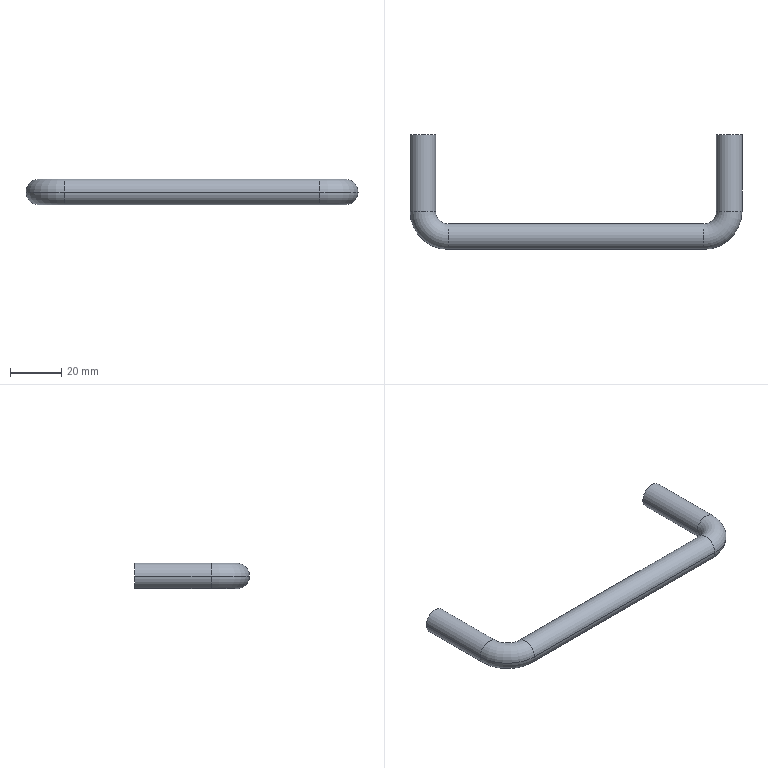Part | SolidWorks | features Sweep 1 | 1 solid | 12 faces | box 130 x 45 x 10 mm | volume 15034 mm3 | cylinder 6 | torus 4 | plane 2 | commonest cylinder face diameters 10 x6
STEP:
#1=CARTESIAN_POINT('',(50.,-5.,0.));
#2=VERTEX_POINT('',#1);
#3=CARTESIAN_POINT('',(50.,5.,0.));
#4=VERTEX_POINT('',#3);
#5=CARTESIAN_POINT('',(50.,0.,0.));
#6=DIRECTION('',(-1.,0.,0.));
#7=DIRECTION('',(0.,0.,-1.));
#8=AXIS2_PLACEMENT_3D('',#5,#6,#7);
#9=CIRCLE('',#8,5.);
#10=EDGE_CURVE('',#2,#4,#9,.T.);
#11=ORIENTED_EDGE('',*,*,#10,.F.);
#12=CARTESIAN_POINT('',(65.,10.,0.));
#13=VERTEX_POINT('',#12);
#14=CARTESIAN_POINT('',(50.,10.,0.));
#15=DIRECTION('',(0.,0.,1.));
#16=DIRECTION('',(1.,0.,0.));
#17=AXIS2_PLACEMENT_3D('',#14,#15,#16);
#18=CIRCLE('',#17,15.);
#19=EDGE_CURVE('',#2,#13,#18,.T.);
#20=ORIENTED_EDGE('',*,*,#19,.T.);
#21=CARTESIAN_POINT('',(55.,10.,0.));
#22=VERTEX_POINT('',#21);
#23=CARTESIAN_POINT('',(60.,10.,0.));
#24=DIRECTION('',(0.,-1.,0.));
#25=DIRECTION('',(0.,0.,-1.));
#26=AXIS2_PLACEMENT_3D('',#23,#24,#25);
#27=CIRCLE('',#26,5.);
#28=EDGE_CURVE('',#13,#22,#27,.T.);
#29=ORIENTED_EDGE('',*,*,#28,.T.);
#30=CARTESIAN_POINT('',(50.,10.,0.));
#31=DIRECTION('',(0.,0.,1.));
#32=DIRECTION('',(1.,0.,0.));
#33=AXIS2_PLACEMENT_3D('',#30,#31,#32);
#34=CIRCLE('',#33,5.);
#35=EDGE_CURVE('',#4,#22,#34,.T.);
#36=ORIENTED_EDGE('',*,*,#35,.F.);
#37=EDGE_LOOP('',(#11,#20,#29,#36));
#38=FACE_OUTER_BOUND('',#37,.T.);
#39=CARTESIAN_POINT('',(50.,10.,0.));
#40=DIRECTION('',(0.,0.,1.));
#41=DIRECTION('',(1.,0.,0.));
#42=AXIS2_PLACEMENT_3D('',#39,#40,#41);
#43=TOROIDAL_SURFACE('',#42,10.,5.);
#44=ADVANCED_FACE('',(#38),#43,.T.);
#45=CARTESIAN_POINT('',(-65.,10.,0.));
#46=VERTEX_POINT('',#45);
#47=CARTESIAN_POINT('',(-55.,10.,0.));
#48=VERTEX_POINT('',#47);
#49=CARTESIAN_POINT('',(-60.,10.,0.));
#50=DIRECTION('',(0.,1.,0.));
#51=DIRECTION('',(0.,0.,-1.));
#52=AXIS2_PLACEMENT_3D('',#49,#50,#51);
#53=CIRCLE('',#52,5.);
#54=EDGE_CURVE('',#46,#48,#53,.T.);
#55=ORIENTED_EDGE('',*,*,#54,.F.);
#56=CARTESIAN_POINT('',(-50.,-5.,0.));
#57=VERTEX_POINT('',#56);
#58=CARTESIAN_POINT('',(-50.,10.,0.));
#59=DIRECTION('',(0.,0.,1.));
#60=DIRECTION('',(1.,0.,0.));
#61=AXIS2_PLACEMENT_3D('',#58,#59,#60);
#62=CIRCLE('',#61,15.);
#63=EDGE_CURVE('',#46,#57,#62,.T.);
#64=ORIENTED_EDGE('',*,*,#63,.T.);
#65=CARTESIAN_POINT('',(-50.,5.,0.));
#66=VERTEX_POINT('',#65);
#67=CARTESIAN_POINT('',(-50.,0.,0.));
#68=DIRECTION('',(-1.,0.,0.));
#69=DIRECTION('',(0.,0.,-1.));
#70=AXIS2_PLACEMENT_3D('',#67,#68,#69);
#71=CIRCLE('',#70,5.);
#72=EDGE_CURVE('',#57,#66,#71,.T.);
#73=ORIENTED_EDGE('',*,*,#72,.T.);
#74=CARTESIAN_POINT('',(-50.,10.,0.));
#75=DIRECTION('',(0.,0.,1.));
#76=DIRECTION('',(1.,0.,0.));
#77=AXIS2_PLACEMENT_3D('',#74,#75,#76);
#78=CIRCLE('',#77,5.);
#79=EDGE_CURVE('',#48,#66,#78,.T.);
#80=ORIENTED_EDGE('',*,*,#79,.F.);
#81=EDGE_LOOP('',(#55,#64,#73,#80));
#82=FACE_OUTER_BOUND('',#81,.T.);
#83=CARTESIAN_POINT('',(-50.,10.,0.));
#84=DIRECTION('',(0.,0.,1.));
#85=DIRECTION('',(1.,0.,0.));
#86=AXIS2_PLACEMENT_3D('',#83,#84,#85);
#87=TOROIDAL_SURFACE('',#86,10.,5.);
#88=ADVANCED_FACE('',(#82),#87,.T.);
#89=ORIENTED_EDGE('',*,*,#28,.F.);
#90=CARTESIAN_POINT('',(65.,40.,0.));
#91=VERTEX_POINT('',#90);
#92=CARTESIAN_POINT('',(65.,10.,0.));
#93=DIRECTION('',(0.,1.,0.));
#94=VECTOR('',#93,1000.);
#95=LINE('',#92,#94);
#96=EDGE_CURVE('',#13,#91,#95,.T.);
#97=ORIENTED_EDGE('',*,*,#96,.T.);
#98=CARTESIAN_POINT('',(55.,40.,0.));
#99=VERTEX_POINT('',#98);
#100=CARTESIAN_POINT('',(60.,40.,0.));
#101=DIRECTION('',(0.,-1.,0.));
#102=DIRECTION('',(0.,0.,-1.));
#103=AXIS2_PLACEMENT_3D('',#100,#101,#102);
#104=CIRCLE('',#103,5.);
#105=EDGE_CURVE('',#91,#99,#104,.T.);
#106=ORIENTED_EDGE('',*,*,#105,.T.);
#107=CARTESIAN_POINT('',(55.,10.,0.));
#108=DIRECTION('',(0.,1.,0.));
#109=VECTOR('',#108,1000.);
#110=LINE('',#107,#109);
#111=EDGE_CURVE('',#22,#99,#110,.T.);
#112=ORIENTED_EDGE('',*,*,#111,.F.);
#113=EDGE_LOOP('',(#89,#97,#106,#112));
#114=FACE_OUTER_BOUND('',#113,.T.);
#115=CARTESIAN_POINT('',(60.,10.,0.));
#116=DIRECTION('',(0.,1.,0.));
#117=DIRECTION('',(-1.,0.,0.));
#118=AXIS2_PLACEMENT_3D('',#115,#116,#117);
#119=CYLINDRICAL_SURFACE('',#118,5.);
#120=ADVANCED_FACE('',(#114),#119,.T.);
#121=ORIENTED_EDGE('',*,*,#72,.F.);
#122=CARTESIAN_POINT('',(-50.,-5.,0.));
#123=DIRECTION('',(1.,0.,0.));
#124=VECTOR('',#123,1000.);
#125=LINE('',#122,#124);
#126=EDGE_CURVE('',#57,#2,#125,.T.);
#127=ORIENTED_EDGE('',*,*,#126,.T.);
#128=ORIENTED_EDGE('',*,*,#10,.T.);
#129=CARTESIAN_POINT('',(-50.,5.,0.));
#130=DIRECTION('',(1.,0.,0.));
#131=VECTOR('',#130,1000.);
#132=LINE('',#129,#131);
#133=EDGE_CURVE('',#66,#4,#132,.T.);
#134=ORIENTED_EDGE('',*,*,#133,.F.);
#135=EDGE_LOOP('',(#121,#127,#128,#134));
#136=FACE_OUTER_BOUND('',#135,.T.);
#137=CARTESIAN_POINT('',(-50.,0.,0.));
#138=DIRECTION('',(1.,0.,0.));
#139=DIRECTION('',(0.,1.,0.));
#140=AXIS2_PLACEMENT_3D('',#137,#138,#139);
#141=CYLINDRICAL_SURFACE('',#140,5.);
#142=ADVANCED_FACE('',(#136),#141,.T.);
#143=CARTESIAN_POINT('',(-65.,40.,0.));
#144=VERTEX_POINT('',#143);
#145=CARTESIAN_POINT('',(-55.,40.,0.));
#146=VERTEX_POINT('',#145);
#147=CARTESIAN_POINT('',(-60.,40.,0.));
#148=DIRECTION('',(0.,1.,0.));
#149=DIRECTION('',(0.,0.,-1.));
#150=AXIS2_PLACEMENT_3D('',#147,#148,#149);
#151=CIRCLE('',#150,5.);
#152=EDGE_CURVE('',#144,#146,#151,.T.);
#153=ORIENTED_EDGE('',*,*,#152,.F.);
#154=CARTESIAN_POINT('',(-65.,40.,0.));
#155=DIRECTION('',(0.,-1.,0.));
#156=VECTOR('',#155,1000.);
#157=LINE('',#154,#156);
#158=EDGE_CURVE('',#144,#46,#157,.T.);
#159=ORIENTED_EDGE('',*,*,#158,.T.);
#160=ORIENTED_EDGE('',*,*,#54,.T.);
#161=CARTESIAN_POINT('',(-55.,40.,0.));
#162=DIRECTION('',(0.,-1.,0.));
#163=VECTOR('',#162,1000.);
#164=LINE('',#161,#163);
#165=EDGE_CURVE('',#146,#48,#164,.T.);
#166=ORIENTED_EDGE('',*,*,#165,.F.);
#167=EDGE_LOOP('',(#153,#159,#160,#166));
#168=FACE_OUTER_BOUND('',#167,.T.);
#169=CARTESIAN_POINT('',(-60.,40.,0.));
#170=DIRECTION('',(0.,-1.,0.));
#171=DIRECTION('',(1.,0.,0.));
#172=AXIS2_PLACEMENT_3D('',#169,#170,#171);
#173=CYLINDRICAL_SURFACE('',#172,5.);
#174=ADVANCED_FACE('',(#168),#173,.T.);
#175=ORIENTED_EDGE('',*,*,#96,.F.);
#176=CARTESIAN_POINT('',(60.,10.,0.));
#177=DIRECTION('',(0.,-1.,0.));
#178=DIRECTION('',(0.,0.,-1.));
#179=AXIS2_PLACEMENT_3D('',#176,#177,#178);
#180=CIRCLE('',#179,5.);
#181=EDGE_CURVE('',#22,#13,#180,.T.);
#182=ORIENTED_EDGE('',*,*,#181,.F.);
#183=ORIENTED_EDGE('',*,*,#111,.T.);
#184=CARTESIAN_POINT('',(60.,40.,0.));
#185=DIRECTION('',(0.,-1.,0.));
#186=DIRECTION('',(0.,0.,-1.));
#187=AXIS2_PLACEMENT_3D('',#184,#185,#186);
#188=CIRCLE('',#187,5.);
#189=EDGE_CURVE('',#99,#91,#188,.T.);
#190=ORIENTED_EDGE('',*,*,#189,.T.);
#191=EDGE_LOOP('',(#175,#182,#183,#190));
#192=FACE_OUTER_BOUND('',#191,.T.);
#193=CARTESIAN_POINT('',(60.,10.,0.));
#194=DIRECTION('',(0.,1.,0.));
#195=DIRECTION('',(-1.,0.,0.));
#196=AXIS2_PLACEMENT_3D('',#193,#194,#195);
#197=CYLINDRICAL_SURFACE('',#196,5.);
#198=ADVANCED_FACE('',(#192),#197,.T.);
#199=ORIENTED_EDGE('',*,*,#19,.F.);
#200=CARTESIAN_POINT('',(50.,0.,0.));
#201=DIRECTION('',(-1.,0.,0.));
#202=DIRECTION('',(0.,0.,-1.));
#203=AXIS2_PLACEMENT_3D('',#200,#201,#202);
#204=CIRCLE('',#203,5.);
#205=EDGE_CURVE('',#4,#2,#204,.T.);
#206=ORIENTED_EDGE('',*,*,#205,.F.);
#207=ORIENTED_EDGE('',*,*,#35,.T.);
#208=ORIENTED_EDGE('',*,*,#181,.T.);
#209=EDGE_LOOP('',(#199,#206,#207,#208));
#210=FACE_OUTER_BOUND('',#209,.T.);
#211=CARTESIAN_POINT('',(50.,10.,0.));
#212=DIRECTION('',(0.,0.,1.));
#213=DIRECTION('',(1.,0.,0.));
#214=AXIS2_PLACEMENT_3D('',#211,#212,#213);
#215=TOROIDAL_SURFACE('',#214,10.,5.);
#216=ADVANCED_FACE('',(#210),#215,.T.);
#217=ORIENTED_EDGE('',*,*,#126,.F.);
#218=CARTESIAN_POINT('',(-50.,0.,0.));
#219=DIRECTION('',(-1.,0.,0.));
#220=DIRECTION('',(0.,0.,-1.));
#221=AXIS2_PLACEMENT_3D('',#218,#219,#220);
#222=CIRCLE('',#221,5.);
#223=EDGE_CURVE('',#66,#57,#222,.T.);
#224=ORIENTED_EDGE('',*,*,#223,.F.);
#225=ORIENTED_EDGE('',*,*,#133,.T.);
#226=ORIENTED_EDGE('',*,*,#205,.T.);
#227=EDGE_LOOP('',(#217,#224,#225,#226));
#228=FACE_OUTER_BOUND('',#227,.T.);
#229=CARTESIAN_POINT('',(-50.,0.,0.));
#230=DIRECTION('',(1.,0.,0.));
#231=DIRECTION('',(0.,1.,0.));
#232=AXIS2_PLACEMENT_3D('',#229,#230,#231);
#233=CYLINDRICAL_SURFACE('',#232,5.);
#234=ADVANCED_FACE('',(#228),#233,.T.);
#235=ORIENTED_EDGE('',*,*,#63,.F.);
#236=CARTESIAN_POINT('',(-60.,10.,0.));
#237=DIRECTION('',(0.,1.,0.));
#238=DIRECTION('',(0.,0.,-1.));
#239=AXIS2_PLACEMENT_3D('',#236,#237,#238);
#240=CIRCLE('',#239,5.);
#241=EDGE_CURVE('',#48,#46,#240,.T.);
#242=ORIENTED_EDGE('',*,*,#241,.F.);
#243=ORIENTED_EDGE('',*,*,#79,.T.);
#244=ORIENTED_EDGE('',*,*,#223,.T.);
#245=EDGE_LOOP('',(#235,#242,#243,#244));
#246=FACE_OUTER_BOUND('',#245,.T.);
#247=CARTESIAN_POINT('',(-50.,10.,0.));
#248=DIRECTION('',(0.,0.,1.));
#249=DIRECTION('',(1.,0.,0.));
#250=AXIS2_PLACEMENT_3D('',#247,#248,#249);
#251=TOROIDAL_SURFACE('',#250,10.,5.);
#252=ADVANCED_FACE('',(#246),#251,.T.);
#253=ORIENTED_EDGE('',*,*,#158,.F.);
#254=CARTESIAN_POINT('',(-60.,40.,0.));
#255=DIRECTION('',(0.,1.,0.));
#256=DIRECTION('',(0.,0.,-1.));
#257=AXIS2_PLACEMENT_3D('',#254,#255,#256);
#258=CIRCLE('',#257,5.);
#259=EDGE_CURVE('',#146,#144,#258,.T.);
#260=ORIENTED_EDGE('',*,*,#259,.F.);
#261=ORIENTED_EDGE('',*,*,#165,.T.);
#262=ORIENTED_EDGE('',*,*,#241,.T.);
#263=EDGE_LOOP('',(#253,#260,#261,#262));
#264=FACE_OUTER_BOUND('',#263,.T.);
#265=CARTESIAN_POINT('',(-60.,40.,0.));
#266=DIRECTION('',(0.,-1.,0.));
#267=DIRECTION('',(1.,0.,0.));
#268=AXIS2_PLACEMENT_3D('',#265,#266,#267);
#269=CYLINDRICAL_SURFACE('',#268,5.);
#270=ADVANCED_FACE('',(#264),#269,.T.);
#271=ORIENTED_EDGE('',*,*,#189,.F.);
#272=ORIENTED_EDGE('',*,*,#105,.F.);
#273=EDGE_LOOP('',(#271,#272));
#274=FACE_OUTER_BOUND('',#273,.T.);
#275=CARTESIAN_POINT('',(60.,40.,0.));
#276=DIRECTION('',(0.,-1.,0.));
#277=DIRECTION('',(0.,0.,-1.));
#278=AXIS2_PLACEMENT_3D('',#275,#276,#277);
#279=PLANE('',#278);
#280=ADVANCED_FACE('',(#274),#279,.F.);
#281=ORIENTED_EDGE('',*,*,#259,.T.);
#282=ORIENTED_EDGE('',*,*,#152,.T.);
#283=EDGE_LOOP('',(#281,#282));
#284=FACE_OUTER_BOUND('',#283,.T.);
#285=CARTESIAN_POINT('',(-60.,40.,0.));
#286=DIRECTION('',(0.,1.,0.));
#287=DIRECTION('',(0.,0.,-1.));
#288=AXIS2_PLACEMENT_3D('',#285,#286,#287);
#289=PLANE('',#288);
#290=ADVANCED_FACE('',(#284),#289,.T.);
#291=CLOSED_SHELL('',(#44,#88,#120,#142,#174,#198,#216,#234,#252,#270,#280,#290));
#292=MANIFOLD_SOLID_BREP('',#291);
#293=CARTESIAN_POINT('',(0.,0.,0.));
#294=DIRECTION('',(0.,0.,1.));
#295=DIRECTION('',(1.,0.,0.));
#296=AXIS2_PLACEMENT_3D('',#293,#294,#295);
#297=(LENGTH_UNIT()NAMED_UNIT(*)SI_UNIT(.MILLI.,.METRE.));
#298=UNCERTAINTY_MEASURE_WITH_UNIT(LENGTH_MEASURE(0.00001),#297,'','');
#299=(NAMED_UNIT(*)PLANE_ANGLE_UNIT()SI_UNIT($,.RADIAN.));
#300=(NAMED_UNIT(*)SI_UNIT($,.STERADIAN.)SOLID_ANGLE_UNIT());
#301=(GEOMETRIC_REPRESENTATION_CONTEXT(3)GLOBAL_UNCERTAINTY_ASSIGNED_CONTEXT((#298))GLOBAL_UNIT_ASSIGNED_CONTEXT((#297,#299,#300))REPRESENTATION_CONTEXT('',''));
#302=ADVANCED_BREP_SHAPE_REPRESENTATION('',(#292,#296),#301);